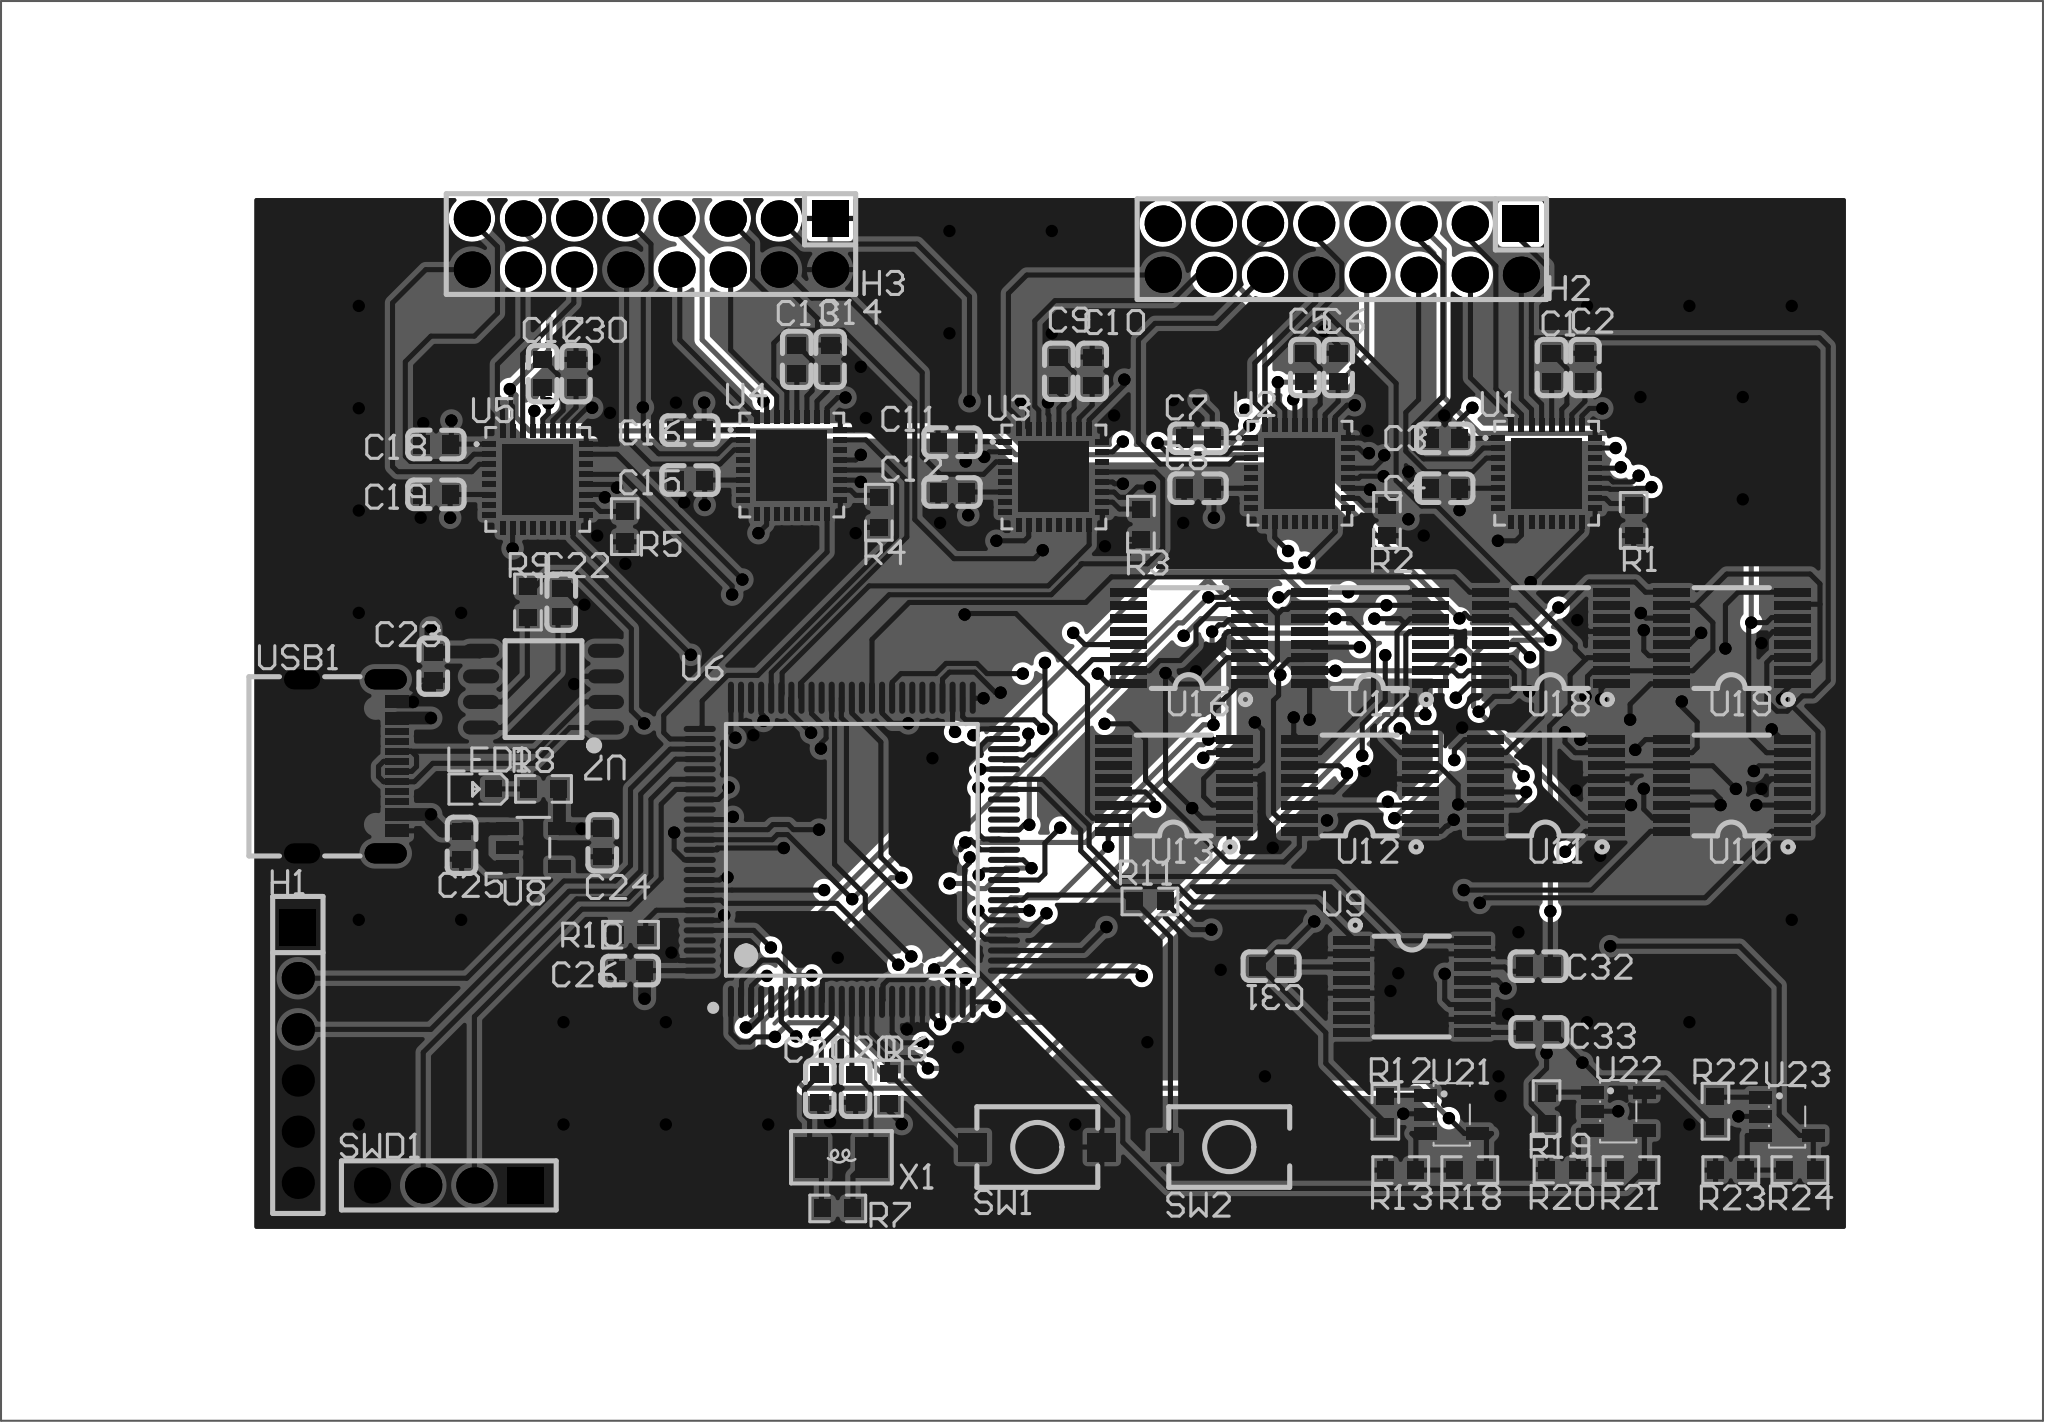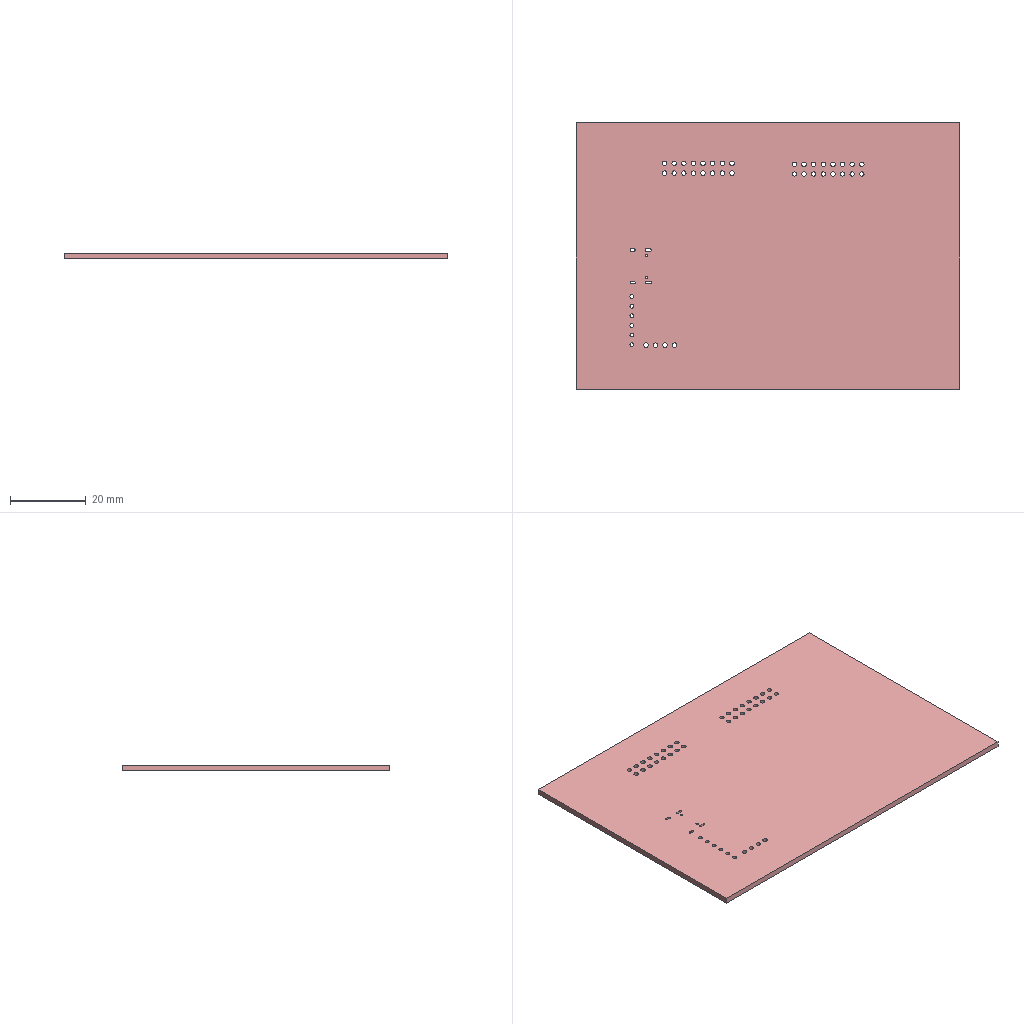Circuit board layout | Altium Designer | box 101.3 x 70.5 x 1.5 mm
Layer stack:
# Altium Designer layer stack of  (unit mm; dielectric type: 0 none, 1 core, 2 prepreg, 3 surface material)
index,name,kind,layer,copper_thickness_mm,dielectric_type,dielectric_thickness_mm,dielectric_material,dielectric_constant
0,Top Paste Mask Layer,other,,,,,,
1,Top Silkscreen Layer,other,,,,,,
2,Top Solder Mask Layer,dielectric,,,3,0,,0
3,Top Layer,copper,Top Layer,0.035,,,,
4,Dielectric1,dielectric,,,3,0.0994,3313 RC57% 4.2mil,0
5,Inner1,copper,Inner1,0.0152,,,,
6,Dielectric2,dielectric,,,3,0.55,0.55mm H/H No copper,0
7,Inner2,copper,Inner2,0.0152,,,,
8,Dielectric3,dielectric,,,3,0.1088,2116 RC54% 4.9mil,0
9,Inner3,copper,Inner3,0.0152,,,,
10,Dielectric4,dielectric,,,3,0.55,0.55mm H/H No copper,0
11,Inner4,copper,Inner4,0.0152,,,,
12,Dielectric5,dielectric,,,3,0.0994,3313 RC57% 4.2mil,0
13,Bottom Layer,copper,Bottom Layer,0.035,,,,
14,Bottom Solder Mask Layer,dielectric,,,3,0,,0
15,Bottom Silkscreen Layer,other,,,,,,
16,Bottom Paste Mask Layer,other,,,,,,
# drill layer pairs: low layer,high layer
drill_pair,Top Layer,Bottom Layer
Part placement:
Designator,Comment,Layer,Footprint,Center-X(mm),Center-Y(mm),Rotation
C23,0.1UF,TopLayer,C0603,91.313,107.315,90
U7,CH340N,TopLayer,SOP-8_150MIL,96.774,106.172,180
C22,0.1UF,TopLayer,C0603,97.663,110.49,90
R9,100R,TopLayer,R0603,96.003,110.499,90
R8,4.7k,TopLayer,R0603,96.774,101.219,0
X1,8MHz,TopLayer,SMD322522,111.561,82.931,180
C21,22pf,TopLayer,C0603,110.49,86.36,90
C20,22pf,TopLayer,C0603,112.268,86.36,90
R7,1M,TopLayer,R0603,111.379,80.391,180
SW1,YTS1C0191ABG00,TopLayer,SW-SMD_L6.0-W4.0-LS7.2,121.285,83.439,180
R6,4.7k,TopLayer,R0603,113.919,86.36,270
R5,470K/1%,TopLayer,R0603,100.808,114.242,90
C19,10nF/25V,TopLayer,C0603,91.44,115.84,0
C18,4.7uF/50V,TopLayer,C0603,91.44,118.314,0
C30,104,TopLayer,C0603,98.389,121.842,90
C17,4.7uF/50V,TopLayer,C0603,96.738,121.842,90
R4,470K/1%,TopLayer,R0603,113.417,114.955,90
C16,10nF/25V,TopLayer,C0603,104.049,119.027,0
C15,4.7uF/50V,TopLayer,C0603,104.049,116.552,0
C14,104,TopLayer,C0603,110.998,122.555,90
C13,4.7uF/50V,TopLayer,C0603,109.347,122.555,90
R3,470K/1%,TopLayer,R0603,126.425,114.361,90
C12,10nF/25V,TopLayer,C0603,117.057,115.958,0
C11,4.7uF/50V,TopLayer,C0603,117.057,118.433,0
C10,104,TopLayer,C0603,124.006,121.961,90
C9,4.7uF/50V,TopLayer,C0603,122.355,121.961,90
R2,470K/1%,TopLayer,R0603,138.635,114.548,90
C8,10nF/25V,TopLayer,C0603,129.268,116.146,0
C7,4.7uF/50V,TopLayer,C0603,129.268,118.621,0
C6,104,TopLayer,C0603,136.217,122.149,90
C5,4.7uF/50V,TopLayer,C0603,134.566,122.149,90
C1,22pf/50V,TopLayer,C0603,146.811,122.149,90
C2,104,TopLayer,C0603,148.462,122.149,90
C4,4.7uF/50V,TopLayer,C0603,141.513,116.146,0
C3,10nF/25V,TopLayer,C0603,141.513,118.621,0
R1,470K/1%,TopLayer,R0603,150.881,114.548,90
C24,106,TopLayer,C0603,99.695,98.552,90
C25,106,TopLayer,C0603,92.71,98.428,90
H2,PZ254V-12-16P,TopLayer,HDR-TH_16P-P2.54-V-M-R2-C8-S2.54,136.398,128.016,180
H3,PZ254V-12-16P,TopLayer,HDR-TH_16P-P2.54-V-M-R2-C8-S2.54,102.108,128.27,180
U1,PCAP01AD,TopLayer,VQFN-32_L5.0-W5.0-P0.50-TL-EP,146.563,116.892,0
U2,PCAP01AD,TopLayer,VQFN-32_L5.0-W5.0-P0.50-TL-EP,134.317,116.892,0
U3,PCAP01AD,TopLayer,VQFN-32_L5.0-W5.0-P0.50-TL-EP,122.107,116.705,0
U4,PCAP01AD,TopLayer,VQFN-32_L5.0-W5.0-P0.50-TL-EP,109.099,117.299,0
U5,PCAP01AD,TopLayer,VQFN-32_L5.0-W5.0-P0.50-TL-EP,96.49,116.586,0
USB1,TYPE-C16PIN,TopLayer,USB-C-SMD_TYPE-C16PIN,87.154,102.339,270
SWD1,A2541HWV-4P,TopLayer,HDR-TH_4P-P2.54-V_A2541HWV-4P,92.075,81.534,180
LED1,19-217/R6C-AL1M2VY/3T,TopLayer,LED0603-RD,93.472,101.219,180
U8,RT9013-3.3GB,TopLayer,SOT-23-5_L2.9-W1.6-P0.94-LS2.8-BL,96.266,98.298,270
C26,100nF,TopLayer,C0603,101.092,92.202,0
C31,500uF,TopLayer,C0603,132.888,92.419,180
C32,500uF,TopLayer,C0603,146.139,92.419,180
C33,500uF,TopLayer,C0603,146.177,89.154,180
R10,10K,TopLayer,R0603,101.092,93.98,180
R11,4.7k,TopLayer,R0603,126.873,95.631,0
R12,10K,TopLayer,R0603,138.557,85.217,90
R13,10K,TopLayer,R0603,139.319,82.296,0
R18,10K,TopLayer,R0603,142.748,82.296,0
R19,10K,TopLayer,R0603,146.558,85.344,90
R20,10K,TopLayer,R0603,147.327,82.322,0
R21,10K,TopLayer,R0603,150.749,82.296,0
R22,10K,TopLayer,R0603,154.94,85.217,90
R23,10K,TopLayer,R0603,155.702,82.296,0
R24,10K,TopLayer,R0603,159.131,82.296,0
SW2,YTS1C0191ABG00,TopLayer,SW-SMD_L6.0-W4.0-LS7.2,130.81,83.439,180
U6,STM32F103VET6,TopLayer,LQFP-100_L14.0-W14.0-P0.50-LS16.0-BL,112.078,98.196,0
U9,TMUX1112PWR,TopLayer,TSSOP-16_L5.0-W4.4-P0.65-LS6.4-TL,139.858,91.403,0
U10,TMUX1112PWR,TopLayer,TSSOP-16_L5.0-W4.4-P0.65-LS6.4-TL,155.75,101.392,180
U11,TMUX1112PWR,TopLayer,TSSOP-16_L5.0-W4.4-P0.65-LS6.4-TL,146.519,101.392,180
U12,TMUX1112PWR,TopLayer,TSSOP-16_L5.0-W4.4-P0.65-LS6.4-TL,137.288,101.392,180
U13,TMUX1112PWR,TopLayer,TSSOP-16_L5.0-W4.4-P0.65-LS6.4-TL,128.057,101.392,180
U16,TMUX1112PWR,TopLayer,TSSOP-16_L5.0-W4.4-P0.65-LS6.4-TL,128.819,108.71,180
U17,TMUX1112PWR,TopLayer,TSSOP-16_L5.0-W4.4-P0.65-LS6.4-TL,137.796,108.71,180
U18,TMUX1112PWR,TopLayer,TSSOP-16_L5.0-W4.4-P0.65-LS6.4-TL,146.773,108.71,180
U19,TMUX1112PWR,TopLayer,TSSOP-16_L5.0-W4.4-P0.65-LS6.4-TL,155.75,108.71,180
U21,LMV321IDBVR,TopLayer,SOT-23-5_L3.0-W1.7-P0.95-LS2.8-BR,141.852,85.061,180
U22,LMV321IDBVR,TopLayer,SOT-23-5_L3.0-W1.7-P0.95-LS2.8-BR,150.114,85.217,180
U23,LMV321IDBVR,TopLayer,SOT-23-5_L3.0-W1.7-P0.95-LS2.8-BR,158.496,84.963,180
H1,,TopLayer,HDR-TH_6P-P2.54-V-F,84.582,88.011,270
Pad and via stacks:
# Altium Designer via and pad stacks of  (unit mm). Each distinct definition once, with the count of objects using it.
# via: kind,start_layer,end_layer,hole_mm,diameter_mm,mode(0 simple;1 top-mid-bottom;2 full stack),diameter_per_layer,count,example_net
# pad: kind,layer,hole_mm,hole_type(0 round;1 square;2 slot),plating,top_size,top_shape(1 round;2 rect;3 octagon;9 rounded rect),mid_size,bottom_size,mode,footprint,size_per_layer,count,example
pad,Top Layer,0,0,plated,0.8x0.9,2,0.8x0.9,0.8x0.9,0,C0603,,60,C23.1
pad,Top Layer,0,0,plated,0.7x1.8,1,0.7x1.8,0.7x1.8,0,SOP-8_150MIL,,8,U7.5
pad,Top Layer,0,0,plated,0.8065x0.864,2,0.8065x0.864,0.8065x0.864,0,R0603,,40,R9.2
pad,Top Layer,0,0,plated,1.6x2,2,1.6x2,1.6x2,0,SMD322522,,2,X1.2
pad,Top Layer,0,0,plated,1.4x1.4,2,1.4x1.4,1.4x1.4,0,SW-SMD_L6.0-W4.0-LS7.2,,4,SW1.1
pad,Top Layer,0,0,plated,0.665x0.28,2,0.665x0.28,0.665x0.28,0,VQFN-32_L5.0-W5.0-P0.50-TL-EP,,80,U1.1
pad,Top Layer,0,0,plated,0.28x0.665,2,0.28x0.665,0.28x0.665,0,VQFN-32_L5.0-W5.0-P0.50-TL-EP,,80,U1.9
pad,Top Layer,0,0,plated,3.5x3.5,2,3.5x3.5,3.5x3.5,0,VQFN-32_L5.0-W5.0-P0.50-TL-EP,,5,U1.33
pad,Top Layer,0,0,plated,0.6x1.15,2,0.6x1.15,0.6x1.15,0,USB-C-SMD_TYPE-C16PIN,,4,USB1.A1B12
pad,Top Layer,0,0,plated,0.3x1.15,2,0.3x1.15,0.3x1.15,0,USB-C-SMD_TYPE-C16PIN,,8,USB1.B5
pad,Top Layer,0,0,plated,0.8x0.8,2,0.8x0.8,0.8x0.8,0,LED0603-RD,,2,LED1.2
pad,Top Layer,0,0,plated,1.1x0.6,2,1.1x0.6,1.1x0.6,0,SOT-23-5_L2.9-W1.6-P0.94-LS2.8-BL,,5,U8.2
pad,Top Layer,0,0,plated,1.6x0.3,1,1.6x0.3,1.6x0.3,0,LQFP-100_L14.0-W14.0-P0.50-LS16.0-BL,,50,U6.100
pad,Top Layer,0,0,plated,0.3x1.6,1,0.3x1.6,0.3x1.6,0,LQFP-100_L14.0-W14.0-P0.50-LS16.0-BL,,50,U6.75
pad,Top Layer,0,0,plated,1.803x0.4064,2,1.803x0.4064,1.803x0.4064,0,TSSOP-16_L5.0-W4.4-P0.65-LS6.4-TL,,144,U9.16
pad,Top Layer,0,0,plated,1.1x0.6,2,1.1x0.6,1.1x0.6,0,SOT-23-5_L3.0-W1.7-P0.95-LS2.8-BR,,15,U21.5
pad,Multi-Layer,1.2,0,plated,1.8x1.8,1,1.8x1.8,1.8x1.8,0,HDR-TH_16P-P2.54-V-M-R2-C8-S2.54,,30,H2.16
pad,Multi-Layer,1.2,0,plated,1.8x1.8,2,1.8x1.8,1.8x1.8,0,HDR-TH_16P-P2.54-V-M-R2-C8-S2.54,,2,H2.1
pad,Multi-Layer,0.6,2,plated,1x1.8,1,1x1.8,1x1.8,0,USB-C-SMD_TYPE-C16PIN,,2,USB1.4
pad,Multi-Layer,0.6,2,plated,1x2.1,1,1x2.1,1x2.1,0,USB-C-SMD_TYPE-C16PIN,,2,USB1.2
pad,Multi-Layer,1.2,0,plated,1.8x1.8,2,1.8x1.8,1.8x1.8,0,HDR-TH_4P-P2.54-V_A2541HWV-4P,,1,SWD1.1
pad,Multi-Layer,1.2,0,plated,1.8x1.8,1,1.8x1.8,1.8x1.8,0,HDR-TH_4P-P2.54-V_A2541HWV-4P,,3,SWD1.2
pad,Multi-Layer,1.02,0,plated,1.6x1.6,1,1.6x1.6,1.6x1.6,0,HDR-TH_6P-P2.54-V-F,,5,H1.6
pad,Multi-Layer,1.02,0,plated,1.8x1.8,2,1.8x1.8,1.8x1.8,0,HDR-TH_6P-P2.54-V-F,,1,H1.1
via,Top Layer,Bottom Layer,0.3048,0.61,0,,275,EC1
Copper pours:
name,layer,net,type(0 solid;1 hatched;2 none)
Bottom Layer-GND,Bottom Layer,GND,0
Top Layer-GND,Top Layer,GND,0
Design rules, without the lines most boards share:
# Altium Designer design rules of  (exported by Altium Designer, unit mm)
# columns: name | kind | enabled | priority | scope1 | scope2 | descriptor | typed fields (field=value)
otherClearance | 52 | enabled | 1 | All | All | Hole To Hole Clearance (Gap=11.8mil) (All),(All) | gap=0.2997
copperRegion | 20 | enabled | 1 | (InNet('GND')) | All | Polygon Connect Rule(Relief Connect )(Conductor Width=10mil) (Relief Angle=90 Angle) (Entries=4) (Air Gap Width=10mil) ((InNet('GND'))),(All) | connect_style(0=relief,1=direct,2=none)=0 relief_conductor_width=0.254 relief_entries=4